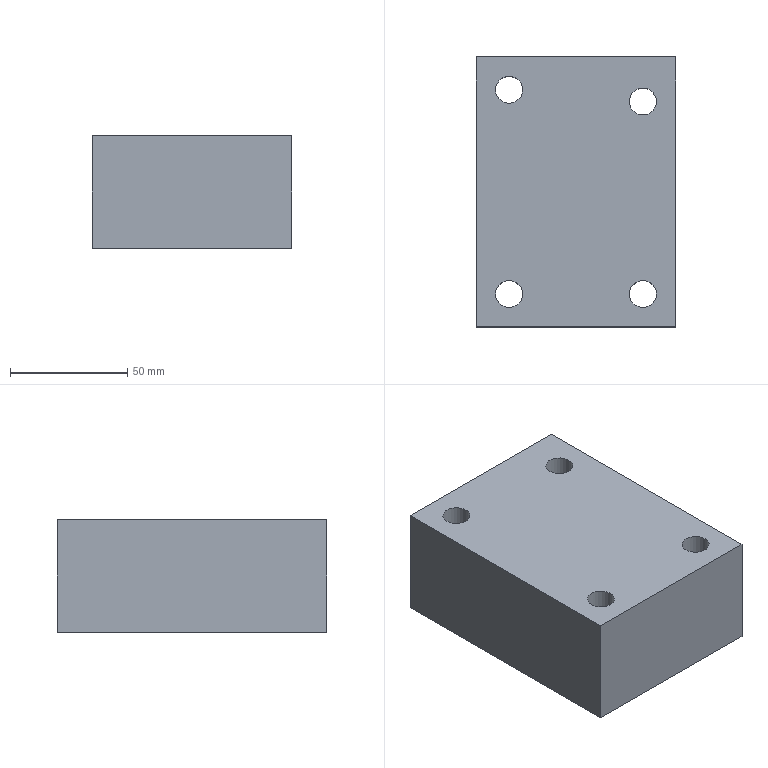Part | NX | features solid 2 | 1 solid | 35 faces | box 85 x 115 x 48 mm | volume 405580 mm3 | cylinder 16 | plane 15 | cone 4 | commonest cylinder face diameters 10 x4 11.509 x4 18.007 x4 8.5 x2 8.506 x2
STEP:
#1=CARTESIAN_POINT('',(1168.789,202.654,50.));
#2=VERTEX_POINT('',#1);
#3=CARTESIAN_POINT('',(1159.786,202.654,50.));
#4=DIRECTION('',(0.,0.,1.));
#5=DIRECTION('',(1.,0.,0.));
#6=AXIS2_PLACEMENT_3D('',#3,#4,#5);
#7=CIRCLE('',#6,9.004);
#8=EDGE_CURVE('',#2,#2,#7,.T.);
#9=ORIENTED_EDGE('',*,*,#8,.T.);
#10=EDGE_LOOP('',(#9));
#11=FACE_BOUND('',#10,.T.);
#12=CARTESIAN_POINT('',(1225.789,115.654,50.));
#13=VERTEX_POINT('',#12);
#14=CARTESIAN_POINT('',(1216.786,115.654,50.));
#15=DIRECTION('',(0.,0.,1.));
#16=DIRECTION('',(1.,0.,0.));
#17=AXIS2_PLACEMENT_3D('',#14,#15,#16);
#18=CIRCLE('',#17,9.004);
#19=EDGE_CURVE('',#13,#13,#18,.T.);
#20=ORIENTED_EDGE('',*,*,#19,.T.);
#21=EDGE_LOOP('',(#20));
#22=FACE_BOUND('',#21,.T.);
#23=CARTESIAN_POINT('',(1230.786,216.654,50.));
#24=VERTEX_POINT('',#23);
#25=CARTESIAN_POINT('',(1145.786,216.654,50.));
#26=VERTEX_POINT('',#25);
#27=CARTESIAN_POINT('',(1188.286,216.654,50.));
#28=DIRECTION('',(-1.,0.,0.));
#29=VECTOR('',#28,1000.);
#30=LINE('',#27,#29);
#31=EDGE_CURVE('',#24,#26,#30,.T.);
#32=ORIENTED_EDGE('',*,*,#31,.F.);
#33=CARTESIAN_POINT('',(1230.786,101.654,50.));
#34=VERTEX_POINT('',#33);
#35=CARTESIAN_POINT('',(1230.786,0.,50.));
#36=DIRECTION('',(0.,-1.,0.));
#37=VECTOR('',#36,1000.);
#38=LINE('',#35,#37);
#39=EDGE_CURVE('',#24,#34,#38,.T.);
#40=ORIENTED_EDGE('',*,*,#39,.T.);
#41=CARTESIAN_POINT('',(1145.786,101.654,50.));
#42=VERTEX_POINT('',#41);
#43=CARTESIAN_POINT('',(1127.,101.654,50.));
#44=DIRECTION('',(-1.,0.,0.));
#45=VECTOR('',#44,1000.);
#46=LINE('',#43,#45);
#47=EDGE_CURVE('',#34,#42,#46,.T.);
#48=ORIENTED_EDGE('',*,*,#47,.T.);
#49=CARTESIAN_POINT('',(1145.786,0.,50.));
#50=DIRECTION('',(0.,1.,0.));
#51=VECTOR('',#50,1000.);
#52=LINE('',#49,#51);
#53=EDGE_CURVE('',#42,#26,#52,.T.);
#54=ORIENTED_EDGE('',*,*,#53,.T.);
#55=EDGE_LOOP('',(#32,#40,#48,#54));
#56=FACE_BOUND('',#55,.T.);
#57=CARTESIAN_POINT('',(1225.789,197.654,50.));
#58=VERTEX_POINT('',#57);
#59=CARTESIAN_POINT('',(1216.786,197.654,50.));
#60=DIRECTION('',(0.,0.,1.));
#61=DIRECTION('',(1.,0.,0.));
#62=AXIS2_PLACEMENT_3D('',#59,#60,#61);
#63=CIRCLE('',#62,9.004);
#64=EDGE_CURVE('',#58,#58,#63,.T.);
#65=ORIENTED_EDGE('',*,*,#64,.T.);
#66=EDGE_LOOP('',(#65));
#67=FACE_BOUND('',#66,.T.);
#68=CARTESIAN_POINT('',(1168.789,115.654,50.));
#69=VERTEX_POINT('',#68);
#70=CARTESIAN_POINT('',(1159.786,115.654,50.));
#71=DIRECTION('',(0.,0.,1.));
#72=DIRECTION('',(1.,0.,0.));
#73=AXIS2_PLACEMENT_3D('',#70,#71,#72);
#74=CIRCLE('',#73,9.004);
#75=EDGE_CURVE('',#69,#69,#74,.T.);
#76=ORIENTED_EDGE('',*,*,#75,.T.);
#77=EDGE_LOOP('',(#76));
#78=FACE_BOUND('',#77,.T.);
#79=CARTESIAN_POINT('',(1156.536,159.154,50.));
#80=VERTEX_POINT('',#79);
#81=CARTESIAN_POINT('',(1160.786,159.154,50.));
#82=DIRECTION('',(0.,0.,-1.));
#83=DIRECTION('',(-1.,0.,0.));
#84=AXIS2_PLACEMENT_3D('',#81,#82,#83);
#85=CIRCLE('',#84,4.25);
#86=EDGE_CURVE('',#80,#80,#85,.T.);
#87=ORIENTED_EDGE('',*,*,#86,.F.);
#88=EDGE_LOOP('',(#87));
#89=FACE_BOUND('',#88,.T.);
#90=CARTESIAN_POINT('',(1211.536,159.154,50.));
#91=VERTEX_POINT('',#90);
#92=CARTESIAN_POINT('',(1215.786,159.154,50.));
#93=DIRECTION('',(0.,0.,-1.));
#94=DIRECTION('',(-1.,0.,0.));
#95=AXIS2_PLACEMENT_3D('',#92,#93,#94);
#96=CIRCLE('',#95,4.25);
#97=EDGE_CURVE('',#91,#91,#96,.T.);
#98=ORIENTED_EDGE('',*,*,#97,.F.);
#99=EDGE_LOOP('',(#98));
#100=FACE_BOUND('',#99,.T.);
#101=CARTESIAN_POINT('',(1206.996,131.014,50.));
#102=VERTEX_POINT('',#101);
#103=CARTESIAN_POINT('',(1199.996,124.014,50.));
#104=VERTEX_POINT('',#103);
#105=CARTESIAN_POINT('',(1203.996,127.014,50.));
#106=DIRECTION('',(0.,0.,-1.));
#107=DIRECTION('',(-1.,0.,0.));
#108=AXIS2_PLACEMENT_3D('',#105,#106,#107);
#109=CIRCLE('',#108,5.);
#110=EDGE_CURVE('',#102,#104,#109,.T.);
#111=ORIENTED_EDGE('',*,*,#110,.F.);
#112=CARTESIAN_POINT('',(1206.996,187.154,50.));
#113=VERTEX_POINT('',#112);
#114=CARTESIAN_POINT('',(1206.996,0.,50.));
#115=DIRECTION('',(0.,1.,0.));
#116=VECTOR('',#115,1000.);
#117=LINE('',#114,#116);
#118=EDGE_CURVE('',#102,#113,#117,.T.);
#119=ORIENTED_EDGE('',*,*,#118,.T.);
#120=CARTESIAN_POINT('',(1199.996,194.154,50.));
#121=VERTEX_POINT('',#120);
#122=CARTESIAN_POINT('',(1203.996,191.154,50.));
#123=DIRECTION('',(0.,0.,-1.));
#124=DIRECTION('',(-1.,0.,0.));
#125=AXIS2_PLACEMENT_3D('',#122,#123,#124);
#126=CIRCLE('',#125,5.);
#127=EDGE_CURVE('',#113,#121,#126,.F.);
#128=ORIENTED_EDGE('',*,*,#127,.T.);
#129=CARTESIAN_POINT('',(1176.576,194.154,50.));
#130=VERTEX_POINT('',#129);
#131=CARTESIAN_POINT('',(1127.,194.154,50.));
#132=DIRECTION('',(-1.,0.,0.));
#133=VECTOR('',#132,1000.);
#134=LINE('',#131,#133);
#135=EDGE_CURVE('',#121,#130,#134,.T.);
#136=ORIENTED_EDGE('',*,*,#135,.T.);
#137=CARTESIAN_POINT('',(1169.576,187.154,50.));
#138=VERTEX_POINT('',#137);
#139=CARTESIAN_POINT('',(1172.576,191.154,50.));
#140=DIRECTION('',(0.,0.,-1.));
#141=DIRECTION('',(-1.,0.,0.));
#142=AXIS2_PLACEMENT_3D('',#139,#140,#141);
#143=CIRCLE('',#142,5.);
#144=EDGE_CURVE('',#138,#130,#143,.T.);
#145=ORIENTED_EDGE('',*,*,#144,.F.);
#146=CARTESIAN_POINT('',(1169.576,131.014,50.));
#147=VERTEX_POINT('',#146);
#148=CARTESIAN_POINT('',(1169.576,0.,50.));
#149=DIRECTION('',(0.,-1.,0.));
#150=VECTOR('',#149,1000.);
#151=LINE('',#148,#150);
#152=EDGE_CURVE('',#138,#147,#151,.T.);
#153=ORIENTED_EDGE('',*,*,#152,.T.);
#154=CARTESIAN_POINT('',(1176.576,124.014,50.));
#155=VERTEX_POINT('',#154);
#156=CARTESIAN_POINT('',(1172.576,127.014,50.));
#157=DIRECTION('',(0.,0.,-1.));
#158=DIRECTION('',(-1.,0.,0.));
#159=AXIS2_PLACEMENT_3D('',#156,#157,#158);
#160=CIRCLE('',#159,5.);
#161=EDGE_CURVE('',#155,#147,#160,.T.);
#162=ORIENTED_EDGE('',*,*,#161,.F.);
#163=CARTESIAN_POINT('',(1127.,124.014,50.));
#164=DIRECTION('',(1.,0.,0.));
#165=VECTOR('',#164,1000.);
#166=LINE('',#163,#165);
#167=EDGE_CURVE('',#155,#104,#166,.T.);
#168=ORIENTED_EDGE('',*,*,#167,.T.);
#169=EDGE_LOOP('',(#111,#119,#128,#136,#145,#153,#162,#168));
#170=FACE_BOUND('',#169,.T.);
#171=CARTESIAN_POINT('',(1127.,0.,50.));
#172=DIRECTION('',(0.,0.,-1.));
#173=DIRECTION('',(-1.,0.,0.));
#174=AXIS2_PLACEMENT_3D('',#171,#172,#173);
#175=PLANE('',#174);
#176=ADVANCED_FACE('',(#11,#22,#56,#67,#78,#89,#100,#170),#175,.T.);
#177=CARTESIAN_POINT('',(1230.786,101.654,98.));
#178=VERTEX_POINT('',#177);
#179=CARTESIAN_POINT('',(1230.786,216.654,98.));
#180=VERTEX_POINT('',#179);
#181=CARTESIAN_POINT('',(1230.786,0.,98.));
#182=DIRECTION('',(0.,1.,0.));
#183=VECTOR('',#182,1000.);
#184=LINE('',#181,#183);
#185=EDGE_CURVE('',#178,#180,#184,.T.);
#186=ORIENTED_EDGE('',*,*,#185,.F.);
#187=CARTESIAN_POINT('',(1230.786,101.654,87.75));
#188=DIRECTION('',(0.,0.,1.));
#189=VECTOR('',#188,1000.);
#190=LINE('',#187,#189);
#191=EDGE_CURVE('',#34,#178,#190,.T.);
#192=ORIENTED_EDGE('',*,*,#191,.F.);
#193=ORIENTED_EDGE('',*,*,#39,.F.);
#194=CARTESIAN_POINT('',(1230.786,216.654,-52.75));
#195=DIRECTION('',(0.,0.,-1.));
#196=VECTOR('',#195,1000.);
#197=LINE('',#194,#196);
#198=EDGE_CURVE('',#180,#24,#197,.T.);
#199=ORIENTED_EDGE('',*,*,#198,.F.);
#200=EDGE_LOOP('',(#186,#192,#193,#199));
#201=FACE_BOUND('',#200,.T.);
#202=CARTESIAN_POINT('',(1230.786,216.654,50.));
#203=DIRECTION('',(1.,0.,0.));
#204=DIRECTION('',(0.,0.,-1.));
#205=AXIS2_PLACEMENT_3D('',#202,#203,#204);
#206=PLANE('',#205);
#207=ADVANCED_FACE('',(#201),#206,.T.);
#208=CARTESIAN_POINT('',(1165.54,202.654,98.));
#209=VERTEX_POINT('',#208);
#210=CARTESIAN_POINT('',(1159.786,202.654,98.));
#211=DIRECTION('',(0.,0.,1.));
#212=DIRECTION('',(1.,0.,0.));
#213=AXIS2_PLACEMENT_3D('',#210,#211,#212);
#214=CIRCLE('',#213,5.755);
#215=EDGE_CURVE('',#209,#209,#214,.T.);
#216=ORIENTED_EDGE('',*,*,#215,.F.);
#217=EDGE_LOOP('',(#216));
#218=FACE_BOUND('',#217,.T.);
#219=CARTESIAN_POINT('',(1165.54,115.654,98.));
#220=VERTEX_POINT('',#219);
#221=CARTESIAN_POINT('',(1159.786,115.654,98.));
#222=DIRECTION('',(0.,0.,1.));
#223=DIRECTION('',(1.,0.,0.));
#224=AXIS2_PLACEMENT_3D('',#221,#222,#223);
#225=CIRCLE('',#224,5.755);
#226=EDGE_CURVE('',#220,#220,#225,.T.);
#227=ORIENTED_EDGE('',*,*,#226,.F.);
#228=EDGE_LOOP('',(#227));
#229=FACE_BOUND('',#228,.T.);
#230=CARTESIAN_POINT('',(1222.54,115.654,98.));
#231=VERTEX_POINT('',#230);
#232=CARTESIAN_POINT('',(1216.786,115.654,98.));
#233=DIRECTION('',(0.,0.,1.));
#234=DIRECTION('',(1.,0.,0.));
#235=AXIS2_PLACEMENT_3D('',#232,#233,#234);
#236=CIRCLE('',#235,5.755);
#237=EDGE_CURVE('',#231,#231,#236,.T.);
#238=ORIENTED_EDGE('',*,*,#237,.F.);
#239=EDGE_LOOP('',(#238));
#240=FACE_BOUND('',#239,.T.);
#241=CARTESIAN_POINT('',(1222.54,197.654,98.));
#242=VERTEX_POINT('',#241);
#243=CARTESIAN_POINT('',(1216.786,197.654,98.));
#244=DIRECTION('',(0.,0.,1.));
#245=DIRECTION('',(1.,0.,0.));
#246=AXIS2_PLACEMENT_3D('',#243,#244,#245);
#247=CIRCLE('',#246,5.755);
#248=EDGE_CURVE('',#242,#242,#247,.T.);
#249=ORIENTED_EDGE('',*,*,#248,.F.);
#250=EDGE_LOOP('',(#249));
#251=FACE_BOUND('',#250,.T.);
#252=CARTESIAN_POINT('',(1145.786,101.654,98.));
#253=VERTEX_POINT('',#252);
#254=CARTESIAN_POINT('',(1188.286,101.654,98.));
#255=DIRECTION('',(-1.,0.,0.));
#256=VECTOR('',#255,1000.);
#257=LINE('',#254,#256);
#258=EDGE_CURVE('',#178,#253,#257,.T.);
#259=ORIENTED_EDGE('',*,*,#258,.F.);
#260=ORIENTED_EDGE('',*,*,#185,.T.);
#261=CARTESIAN_POINT('',(1145.786,216.654,98.));
#262=VERTEX_POINT('',#261);
#263=CARTESIAN_POINT('',(1188.286,216.654,98.));
#264=DIRECTION('',(1.,0.,0.));
#265=VECTOR('',#264,1000.);
#266=LINE('',#263,#265);
#267=EDGE_CURVE('',#262,#180,#266,.T.);
#268=ORIENTED_EDGE('',*,*,#267,.F.);
#269=CARTESIAN_POINT('',(1145.786,0.,98.));
#270=DIRECTION('',(0.,-1.,0.));
#271=VECTOR('',#270,1000.);
#272=LINE('',#269,#271);
#273=EDGE_CURVE('',#262,#253,#272,.T.);
#274=ORIENTED_EDGE('',*,*,#273,.T.);
#275=EDGE_LOOP('',(#259,#260,#268,#274));
#276=FACE_BOUND('',#275,.T.);
#277=CARTESIAN_POINT('',(835.5,0.,98.));
#278=DIRECTION('',(0.,0.,1.));
#279=DIRECTION('',(1.,0.,0.));
#280=AXIS2_PLACEMENT_3D('',#277,#278,#279);
#281=PLANE('',#280);
#282=ADVANCED_FACE('',(#218,#229,#240,#251,#276),#281,.T.);
#283=ORIENTED_EDGE('',*,*,#47,.F.);
#284=ORIENTED_EDGE('',*,*,#191,.T.);
#285=ORIENTED_EDGE('',*,*,#258,.T.);
#286=CARTESIAN_POINT('',(1145.786,101.654,87.75));
#287=DIRECTION('',(0.,0.,-1.));
#288=VECTOR('',#287,1000.);
#289=LINE('',#286,#288);
#290=EDGE_CURVE('',#253,#42,#289,.T.);
#291=ORIENTED_EDGE('',*,*,#290,.T.);
#292=EDGE_LOOP('',(#283,#284,#285,#291));
#293=FACE_BOUND('',#292,.T.);
#294=CARTESIAN_POINT('',(1188.286,101.654,87.75));
#295=DIRECTION('',(0.,-1.,0.));
#296=DIRECTION('',(0.,0.,-1.));
#297=AXIS2_PLACEMENT_3D('',#294,#295,#296);
#298=PLANE('',#297);
#299=ADVANCED_FACE('',(#293),#298,.T.);
#300=ORIENTED_EDGE('',*,*,#267,.T.);
#301=ORIENTED_EDGE('',*,*,#198,.T.);
#302=ORIENTED_EDGE('',*,*,#31,.T.);
#303=CARTESIAN_POINT('',(1145.786,216.654,-52.75));
#304=DIRECTION('',(0.,0.,1.));
#305=VECTOR('',#304,1000.);
#306=LINE('',#303,#305);
#307=EDGE_CURVE('',#26,#262,#306,.T.);
#308=ORIENTED_EDGE('',*,*,#307,.T.);
#309=EDGE_LOOP('',(#300,#301,#302,#308));
#310=FACE_BOUND('',#309,.T.);
#311=CARTESIAN_POINT('',(1188.286,216.654,-52.75));
#312=DIRECTION('',(0.,1.,0.));
#313=DIRECTION('',(0.,0.,1.));
#314=AXIS2_PLACEMENT_3D('',#311,#312,#313);
#315=PLANE('',#314);
#316=ADVANCED_FACE('',(#310),#315,.T.);
#317=ORIENTED_EDGE('',*,*,#273,.F.);
#318=ORIENTED_EDGE('',*,*,#307,.F.);
#319=ORIENTED_EDGE('',*,*,#53,.F.);
#320=ORIENTED_EDGE('',*,*,#290,.F.);
#321=EDGE_LOOP('',(#317,#318,#319,#320));
#322=FACE_BOUND('',#321,.T.);
#323=CARTESIAN_POINT('',(1145.786,216.654,50.));
#324=DIRECTION('',(-1.,0.,0.));
#325=DIRECTION('',(0.,0.,1.));
#326=AXIS2_PLACEMENT_3D('',#323,#324,#325);
#327=PLANE('',#326);
#328=ADVANCED_FACE('',(#322),#327,.T.);
#329=ORIENTED_EDGE('',*,*,#248,.T.);
#330=EDGE_LOOP('',(#329));
#331=FACE_BOUND('',#330,.T.);
#332=CARTESIAN_POINT('',(1222.54,197.654,68.));
#333=VERTEX_POINT('',#332);
#334=CARTESIAN_POINT('',(1216.786,197.654,68.));
#335=DIRECTION('',(0.,0.,1.));
#336=DIRECTION('',(1.,0.,0.));
#337=AXIS2_PLACEMENT_3D('',#334,#335,#336);
#338=CIRCLE('',#337,5.755);
#339=EDGE_CURVE('',#333,#333,#338,.T.);
#340=ORIENTED_EDGE('',*,*,#339,.F.);
#341=EDGE_LOOP('',(#340));
#342=FACE_BOUND('',#341,.T.);
#343=CARTESIAN_POINT('',(1216.786,197.654,45.));
#344=DIRECTION('',(0.,0.,1.));
#345=DIRECTION('',(1.,0.,0.));
#346=AXIS2_PLACEMENT_3D('',#343,#344,#345);
#347=CYLINDRICAL_SURFACE('',#346,5.755);
#348=ADVANCED_FACE('',(#331,#342),#347,.F.);
#349=ORIENTED_EDGE('',*,*,#339,.T.);
#350=EDGE_LOOP('',(#349));
#351=FACE_BOUND('',#350,.T.);
#352=CARTESIAN_POINT('',(1225.789,197.654,68.));
#353=VERTEX_POINT('',#352);
#354=CARTESIAN_POINT('',(1216.786,197.654,68.));
#355=DIRECTION('',(0.,0.,-1.));
#356=DIRECTION('',(1.,0.,0.));
#357=AXIS2_PLACEMENT_3D('',#354,#355,#356);
#358=CIRCLE('',#357,9.004);
#359=EDGE_CURVE('',#353,#353,#358,.F.);
#360=ORIENTED_EDGE('',*,*,#359,.F.);
#361=EDGE_LOOP('',(#360));
#362=FACE_BOUND('',#361,.T.);
#363=CARTESIAN_POINT('',(1216.786,197.654,68.));
#364=DIRECTION('',(0.,0.,1.));
#365=DIRECTION('',(1.,0.,0.));
#366=AXIS2_PLACEMENT_3D('',#363,#364,#365);
#367=PLANE('',#366);
#368=ADVANCED_FACE('',(#351,#362),#367,.F.);
#369=ORIENTED_EDGE('',*,*,#359,.T.);
#370=EDGE_LOOP('',(#369));
#371=FACE_BOUND('',#370,.T.);
#372=ORIENTED_EDGE('',*,*,#64,.F.);
#373=EDGE_LOOP('',(#372));
#374=FACE_BOUND('',#373,.T.);
#375=CARTESIAN_POINT('',(1216.786,197.654,50.));
#376=DIRECTION('',(0.,0.,1.));
#377=DIRECTION('',(1.,0.,0.));
#378=AXIS2_PLACEMENT_3D('',#375,#376,#377);
#379=CYLINDRICAL_SURFACE('',#378,9.004);
#380=ADVANCED_FACE('',(#371,#374),#379,.F.);
#381=ORIENTED_EDGE('',*,*,#237,.T.);
#382=EDGE_LOOP('',(#381));
#383=FACE_BOUND('',#382,.T.);
#384=CARTESIAN_POINT('',(1222.54,115.654,68.));
#385=VERTEX_POINT('',#384);
#386=CARTESIAN_POINT('',(1216.786,115.654,68.));
#387=DIRECTION('',(0.,0.,1.));
#388=DIRECTION('',(1.,0.,0.));
#389=AXIS2_PLACEMENT_3D('',#386,#387,#388);
#390=CIRCLE('',#389,5.755);
#391=EDGE_CURVE('',#385,#385,#390,.T.);
#392=ORIENTED_EDGE('',*,*,#391,.F.);
#393=EDGE_LOOP('',(#392));
#394=FACE_BOUND('',#393,.T.);
#395=CARTESIAN_POINT('',(1216.786,115.654,45.));
#396=DIRECTION('',(0.,0.,1.));
#397=DIRECTION('',(1.,0.,0.));
#398=AXIS2_PLACEMENT_3D('',#395,#396,#397);
#399=CYLINDRICAL_SURFACE('',#398,5.755);
#400=ADVANCED_FACE('',(#383,#394),#399,.F.);
#401=ORIENTED_EDGE('',*,*,#391,.T.);
#402=EDGE_LOOP('',(#401));
#403=FACE_BOUND('',#402,.T.);
#404=CARTESIAN_POINT('',(1225.789,115.654,68.));
#405=VERTEX_POINT('',#404);
#406=CARTESIAN_POINT('',(1216.786,115.654,68.));
#407=DIRECTION('',(0.,0.,-1.));
#408=DIRECTION('',(1.,0.,0.));
#409=AXIS2_PLACEMENT_3D('',#406,#407,#408);
#410=CIRCLE('',#409,9.004);
#411=EDGE_CURVE('',#405,#405,#410,.F.);
#412=ORIENTED_EDGE('',*,*,#411,.F.);
#413=EDGE_LOOP('',(#412));
#414=FACE_BOUND('',#413,.T.);
#415=CARTESIAN_POINT('',(1216.786,115.654,68.));
#416=DIRECTION('',(0.,0.,1.));
#417=DIRECTION('',(1.,0.,0.));
#418=AXIS2_PLACEMENT_3D('',#415,#416,#417);
#419=PLANE('',#418);
#420=ADVANCED_FACE('',(#403,#414),#419,.F.);
#421=ORIENTED_EDGE('',*,*,#411,.T.);
#422=EDGE_LOOP('',(#421));
#423=FACE_BOUND('',#422,.T.);
#424=ORIENTED_EDGE('',*,*,#19,.F.);
#425=EDGE_LOOP('',(#424));
#426=FACE_BOUND('',#425,.T.);
#427=CARTESIAN_POINT('',(1216.786,115.654,50.));
#428=DIRECTION('',(0.,0.,1.));
#429=DIRECTION('',(1.,0.,0.));
#430=AXIS2_PLACEMENT_3D('',#427,#428,#429);
#431=CYLINDRICAL_SURFACE('',#430,9.004);
#432=ADVANCED_FACE('',(#423,#426),#431,.F.);
#433=ORIENTED_EDGE('',*,*,#226,.T.);
#434=EDGE_LOOP('',(#433));
#435=FACE_BOUND('',#434,.T.);
#436=CARTESIAN_POINT('',(1165.54,115.654,68.));
#437=VERTEX_POINT('',#436);
#438=CARTESIAN_POINT('',(1159.786,115.654,68.));
#439=DIRECTION('',(0.,0.,1.));
#440=DIRECTION('',(1.,0.,0.));
#441=AXIS2_PLACEMENT_3D('',#438,#439,#440);
#442=CIRCLE('',#441,5.755);
#443=EDGE_CURVE('',#437,#437,#442,.T.);
#444=ORIENTED_EDGE('',*,*,#443,.F.);
#445=EDGE_LOOP('',(#444));
#446=FACE_BOUND('',#445,.T.);
#447=CARTESIAN_POINT('',(1159.786,115.654,45.));
#448=DIRECTION('',(0.,0.,1.));
#449=DIRECTION('',(1.,0.,0.));
#450=AXIS2_PLACEMENT_3D('',#447,#448,#449);
#451=CYLINDRICAL_SURFACE('',#450,5.755);
#452=ADVANCED_FACE('',(#435,#446),#451,.F.);
#453=ORIENTED_EDGE('',*,*,#443,.T.);
#454=EDGE_LOOP('',(#453));
#455=FACE_BOUND('',#454,.T.);
#456=CARTESIAN_POINT('',(1168.789,115.654,68.));
#457=VERTEX_POINT('',#456);
#458=CARTESIAN_POINT('',(1159.786,115.654,68.));
#459=DIRECTION('',(0.,0.,-1.));
#460=DIRECTION('',(1.,0.,0.));
#461=AXIS2_PLACEMENT_3D('',#458,#459,#460);
#462=CIRCLE('',#461,9.004);
#463=EDGE_CURVE('',#457,#457,#462,.F.);
#464=ORIENTED_EDGE('',*,*,#463,.F.);
#465=EDGE_LOOP('',(#464));
#466=FACE_BOUND('',#465,.T.);
#467=CARTESIAN_POINT('',(1159.786,115.654,68.));
#468=DIRECTION('',(0.,0.,1.));
#469=DIRECTION('',(1.,0.,0.));
#470=AXIS2_PLACEMENT_3D('',#467,#468,#469);
#471=PLANE('',#470);
#472=ADVANCED_FACE('',(#455,#466),#471,.F.);
#473=ORIENTED_EDGE('',*,*,#463,.T.);
#474=EDGE_LOOP('',(#473));
#475=FACE_BOUND('',#474,.T.);
#476=ORIENTED_EDGE('',*,*,#75,.F.);
#477=EDGE_LOOP('',(#476));
#478=FACE_BOUND('',#477,.T.);
#479=CARTESIAN_POINT('',(1159.786,115.654,50.));
#480=DIRECTION('',(0.,0.,1.));
#481=DIRECTION('',(1.,0.,0.));
#482=AXIS2_PLACEMENT_3D('',#479,#480,#481);
#483=CYLINDRICAL_SURFACE('',#482,9.004);
#484=ADVANCED_FACE('',(#475,#478),#483,.F.);
#485=ORIENTED_EDGE('',*,*,#215,.T.);
#486=EDGE_LOOP('',(#485));
#487=FACE_BOUND('',#486,.T.);
#488=CARTESIAN_POINT('',(1165.54,202.654,68.));
#489=VERTEX_POINT('',#488);
#490=CARTESIAN_POINT('',(1159.786,202.654,68.));
#491=DIRECTION('',(0.,0.,1.));
#492=DIRECTION('',(1.,0.,0.));
#493=AXIS2_PLACEMENT_3D('',#490,#491,#492);
#494=CIRCLE('',#493,5.755);
#495=EDGE_CURVE('',#489,#489,#494,.T.);
#496=ORIENTED_EDGE('',*,*,#495,.F.);
#497=EDGE_LOOP('',(#496));
#498=FACE_BOUND('',#497,.T.);
#499=CARTESIAN_POINT('',(1159.786,202.654,45.));
#500=DIRECTION('',(0.,0.,1.));
#501=DIRECTION('',(1.,0.,0.));
#502=AXIS2_PLACEMENT_3D('',#499,#500,#501);
#503=CYLINDRICAL_SURFACE('',#502,5.755);
#504=ADVANCED_FACE('',(#487,#498),#503,.F.);
#505=ORIENTED_EDGE('',*,*,#495,.T.);
#506=EDGE_LOOP('',(#505));
#507=FACE_BOUND('',#506,.T.);
#508=CARTESIAN_POINT('',(1168.789,202.654,68.));
#509=VERTEX_POINT('',#508);
#510=CARTESIAN_POINT('',(1159.786,202.654,68.));
#511=DIRECTION('',(0.,0.,-1.));
#512=DIRECTION('',(1.,0.,0.));
#513=AXIS2_PLACEMENT_3D('',#510,#511,#512);
#514=CIRCLE('',#513,9.004);
#515=EDGE_CURVE('',#509,#509,#514,.F.);
#516=ORIENTED_EDGE('',*,*,#515,.F.);
#517=EDGE_LOOP('',(#516));
#518=FACE_BOUND('',#517,.T.);
#519=CARTESIAN_POINT('',(1159.786,202.654,68.));
#520=DIRECTION('',(0.,0.,1.));
#521=DIRECTION('',(1.,0.,0.));
#522=AXIS2_PLACEMENT_3D('',#519,#520,#521);
#523=PLANE('',#522);
#524=ADVANCED_FACE('',(#507,#518),#523,.F.);
#525=ORIENTED_EDGE('',*,*,#515,.T.);
#526=EDGE_LOOP('',(#525));
#527=FACE_BOUND('',#526,.T.);
#528=ORIENTED_EDGE('',*,*,#8,.F.);
#529=EDGE_LOOP('',(#528));
#530=FACE_BOUND('',#529,.T.);
#531=CARTESIAN_POINT('',(1159.786,202.654,50.));
#532=DIRECTION('',(0.,0.,1.));
#533=DIRECTION('',(1.,0.,0.));
#534=AXIS2_PLACEMENT_3D('',#531,#532,#533);
#535=CYLINDRICAL_SURFACE('',#534,9.004);
#536=ADVANCED_FACE('',(#527,#530),#535,.F.);
#537=CARTESIAN_POINT('',(1156.536,159.154,70.));
#538=VERTEX_POINT('',#537);
#539=CARTESIAN_POINT('',(1160.786,159.154,70.));
#540=DIRECTION('',(0.,0.,-1.));
#541=DIRECTION('',(-1.,0.,0.));
#542=AXIS2_PLACEMENT_3D('',#539,#540,#541);
#543=CIRCLE('',#542,4.25);
#544=EDGE_CURVE('',#538,#538,#543,.F.);
#545=ORIENTED_EDGE('',*,*,#544,.F.);
#546=EDGE_LOOP('',(#545));
#547=FACE_BOUND('',#546,.T.);
#548=CARTESIAN_POINT('',(1160.786,159.154,72.554));
#549=VERTEX_POINT('',#548);
#550=VERTEX_LOOP('',#549);
#551=FACE_BOUND('',#550,.T.);
#552=CARTESIAN_POINT('',(1160.786,159.154,70.));
#553=DIRECTION('',(0.,0.,-1.));
#554=DIRECTION('',(1.,0.,0.));
#555=AXIS2_PLACEMENT_3D('',#552,#553,#554);
#556=CONICAL_SURFACE('',#555,4.25,1.03);
#557=ADVANCED_FACE('',(#547,#551),#556,.F.);
#558=ORIENTED_EDGE('',*,*,#86,.T.);
#559=EDGE_LOOP('',(#558));
#560=FACE_BOUND('',#559,.T.);
#561=ORIENTED_EDGE('',*,*,#544,.T.);
#562=EDGE_LOOP('',(#561));
#563=FACE_BOUND('',#562,.T.);
#564=CARTESIAN_POINT('',(1160.786,159.154,50.));
#565=DIRECTION('',(0.,0.,1.));
#566=DIRECTION('',(-1.,0.,0.));
#567=AXIS2_PLACEMENT_3D('',#564,#565,#566);
#568=CYLINDRICAL_SURFACE('',#567,4.25);
#569=ADVANCED_FACE('',(#560,#563),#568,.F.);
#570=CARTESIAN_POINT('',(1220.036,159.154,70.));
#571=VERTEX_POINT('',#570);
#572=CARTESIAN_POINT('',(1215.786,159.154,70.));
#573=DIRECTION('',(0.,0.,1.));
#574=DIRECTION('',(1.,0.,0.));
#575=AXIS2_PLACEMENT_3D('',#572,#573,#574);
#576=CIRCLE('',#575,4.25);
#577=EDGE_CURVE('',#571,#571,#576,.F.);
#578=ORIENTED_EDGE('',*,*,#577,.T.);
#579=EDGE_LOOP('',(#578));
#580=FACE_BOUND('',#579,.T.);
#581=CARTESIAN_POINT('',(1215.786,159.154,72.554));
#582=VERTEX_POINT('',#581);
#583=VERTEX_LOOP('',#582);
#584=FACE_BOUND('',#583,.T.);
#585=CARTESIAN_POINT('',(1215.786,159.154,70.));
#586=DIRECTION('',(0.,0.,-1.));
#587=DIRECTION('',(-1.,0.,0.));
#588=AXIS2_PLACEMENT_3D('',#585,#586,#587);
#589=CONICAL_SURFACE('',#588,4.25,1.03);
#590=ADVANCED_FACE('',(#580,#584),#589,.F.);
#591=ORIENTED_EDGE('',*,*,#97,.T.);
#592=EDGE_LOOP('',(#591));
#593=FACE_BOUND('',#592,.T.);
#594=ORIENTED_EDGE('',*,*,#577,.F.);
#595=EDGE_LOOP('',(#594));
#596=FACE_BOUND('',#595,.T.);
#597=CARTESIAN_POINT('',(1215.786,159.154,50.));
#598=DIRECTION('',(0.,0.,1.));
#599=DIRECTION('',(1.,0.,0.));
#600=AXIS2_PLACEMENT_3D('',#597,#598,#599);
#601=CYLINDRICAL_SURFACE('',#600,4.25);
#602=ADVANCED_FACE('',(#593,#596),#601,.F.);
#603=CARTESIAN_POINT('',(1206.996,131.014,60.));
#604=VERTEX_POINT('',#603);
#605=CARTESIAN_POINT('',(1206.996,131.014,-87.));
#606=DIRECTION('',(0.,0.,1.));
#607=VECTOR('',#606,1000.);
#608=LINE('',#605,#607);
#609=EDGE_CURVE('',#604,#102,#608,.F.);
#610=ORIENTED_EDGE('',*,*,#609,.F.);
#611=CARTESIAN_POINT('',(1206.996,187.154,60.));
#612=VERTEX_POINT('',#611);
#613=CARTESIAN_POINT('',(1206.996,0.,60.));
#614=DIRECTION('',(0.,1.,0.));
#615=VECTOR('',#614,1000.);
#616=LINE('',#613,#615);
#617=EDGE_CURVE('',#612,#604,#616,.F.);
#618=ORIENTED_EDGE('',*,*,#617,.F.);
#619=CARTESIAN_POINT('',(1206.996,187.154,-87.));
#620=DIRECTION('',(0.,0.,1.));
#621=VECTOR('',#620,1000.);
#622=LINE('',#619,#621);
#623=EDGE_CURVE('',#612,#113,#622,.F.);
#624=ORIENTED_EDGE('',*,*,#623,.T.);
#625=ORIENTED_EDGE('',*,*,#118,.F.);
#626=EDGE_LOOP('',(#610,#618,#624,#625));
#627=FACE_BOUND('',#626,.T.);
#628=CARTESIAN_POINT('',(1206.996,0.,-87.));
#629=DIRECTION('',(-1.,0.,0.));
#630=DIRECTION('',(0.,0.,1.));
#631=AXIS2_PLACEMENT_3D('',#628,#629,#630);
#632=PLANE('',#631);
#633=ADVANCED_FACE('',(#627),#632,.T.);
#634=ORIENTED_EDGE('',*,*,#110,.T.);
#635=CARTESIAN_POINT('',(1199.996,124.014,60.));
#636=VERTEX_POINT('',#635);
#637=CARTESIAN_POINT('',(1199.996,124.014,-87.));
#638=DIRECTION('',(0.,0.,1.));
#639=VECTOR('',#638,1000.);
#640=LINE('',#637,#639);
#641=EDGE_CURVE('',#636,#104,#640,.F.);
#642=ORIENTED_EDGE('',*,*,#641,.F.);
#643=CARTESIAN_POINT('',(1203.996,127.014,60.));
#644=DIRECTION('',(0.,0.,1.));
#645=DIRECTION('',(1.,0.,0.));
#646=AXIS2_PLACEMENT_3D('',#643,#644,#645);
#647=CIRCLE('',#646,5.);
#648=EDGE_CURVE('',#636,#604,#647,.T.);
#649=ORIENTED_EDGE('',*,*,#648,.T.);
#650=ORIENTED_EDGE('',*,*,#609,.T.);
#651=EDGE_LOOP('',(#634,#642,#649,#650));
#652=FACE_BOUND('',#651,.T.);
#653=CARTESIAN_POINT('',(1203.996,127.014,-87.));
#654=DIRECTION('',(0.,0.,1.));
#655=DIRECTION('',(1.,0.,0.));
#656=AXIS2_PLACEMENT_3D('',#653,#654,#655);
#657=CYLINDRICAL_SURFACE('',#656,5.);
#658=ADVANCED_FACE('',(#652),#657,.F.);
#659=CARTESIAN_POINT('',(1176.576,124.014,60.));
#660=VERTEX_POINT('',#659);
#661=CARTESIAN_POINT('',(1176.576,124.014,-87.));
#662=DIRECTION('',(0.,0.,1.));
#663=VECTOR('',#662,1000.);
#664=LINE('',#661,#663);
#665=EDGE_CURVE('',#660,#155,#664,.F.);
#666=ORIENTED_EDGE('',*,*,#665,.F.);
#667=CARTESIAN_POINT('',(268.879,124.014,60.));
#668=DIRECTION('',(1.,0.,0.));
#669=VECTOR('',#668,1000.);
#670=LINE('',#667,#669);
#671=EDGE_CURVE('',#636,#660,#670,.F.);
#672=ORIENTED_EDGE('',*,*,#671,.F.);
#673=ORIENTED_EDGE('',*,*,#641,.T.);
#674=ORIENTED_EDGE('',*,*,#167,.F.);
#675=EDGE_LOOP('',(#666,#672,#673,#674));
#676=FACE_BOUND('',#675,.T.);
#677=CARTESIAN_POINT('',(268.879,124.014,-87.));
#678=DIRECTION('',(0.,1.,0.));
#679=DIRECTION('',(0.,0.,1.));
#680=AXIS2_PLACEMENT_3D('',#677,#678,#679);
#681=PLANE('',#680);
#682=ADVANCED_FACE('',(#676),#681,.T.);
#683=ORIENTED_EDGE('',*,*,#161,.T.);
#684=CARTESIAN_POINT('',(1169.576,131.014,60.));
#685=VERTEX_POINT('',#684);
#686=CARTESIAN_POINT('',(1169.576,131.014,-87.));
#687=DIRECTION('',(0.,0.,1.));
#688=VECTOR('',#687,1000.);
#689=LINE('',#686,#688);
#690=EDGE_CURVE('',#685,#147,#689,.F.);
#691=ORIENTED_EDGE('',*,*,#690,.F.);
#692=CARTESIAN_POINT('',(1172.576,127.014,60.));
#693=DIRECTION('',(0.,0.,1.));
#694=DIRECTION('',(1.,0.,0.));
#695=AXIS2_PLACEMENT_3D('',#692,#693,#694);
#696=CIRCLE('',#695,5.);
#697=EDGE_CURVE('',#685,#660,#696,.T.);
#698=ORIENTED_EDGE('',*,*,#697,.T.);
#699=ORIENTED_EDGE('',*,*,#665,.T.);
#700=EDGE_LOOP('',(#683,#691,#698,#699));
#701=FACE_BOUND('',#700,.T.);
#702=CARTESIAN_POINT('',(1172.576,127.014,-87.));
#703=DIRECTION('',(0.,0.,1.));
#704=DIRECTION('',(1.,0.,0.));
#705=AXIS2_PLACEMENT_3D('',#702,#703,#704);
#706=CYLINDRICAL_SURFACE('',#705,5.);
#707=ADVANCED_FACE('',(#701),#706,.F.);
#708=CARTESIAN_POINT('',(1169.576,187.154,60.));
#709=VERTEX_POINT('',#708);
#710=CARTESIAN_POINT('',(1169.576,187.154,-87.));
#711=DIRECTION('',(0.,0.,1.));
#712=VECTOR('',#711,1000.);
#713=LINE('',#710,#712);
#714=EDGE_CURVE('',#709,#138,#713,.F.);
#715=ORIENTED_EDGE('',*,*,#714,.F.);
#716=CARTESIAN_POINT('',(1169.576,0.,60.));
#717=DIRECTION('',(0.,-1.,0.));
#718=VECTOR('',#717,1000.);
#719=LINE('',#716,#718);
#720=EDGE_CURVE('',#685,#709,#719,.F.);
#721=ORIENTED_EDGE('',*,*,#720,.F.);
#722=ORIENTED_EDGE('',*,*,#690,.T.);
#723=ORIENTED_EDGE('',*,*,#152,.F.);
#724=EDGE_LOOP('',(#715,#721,#722,#723));
#725=FACE_BOUND('',#724,.T.);
#726=CARTESIAN_POINT('',(1169.576,0.,-87.));
#727=DIRECTION('',(1.,0.,0.));
#728=DIRECTION('',(0.,0.,-1.));
#729=AXIS2_PLACEMENT_3D('',#726,#727,#728);
#730=PLANE('',#729);
#731=ADVANCED_FACE('',(#725),#730,.T.);
#732=ORIENTED_EDGE('',*,*,#144,.T.);
#733=CARTESIAN_POINT('',(1176.576,194.154,60.));
#734=VERTEX_POINT('',#733);
#735=CARTESIAN_POINT('',(1176.576,194.154,-87.));
#736=DIRECTION('',(0.,0.,1.));
#737=VECTOR('',#736,1000.);
#738=LINE('',#735,#737);
#739=EDGE_CURVE('',#734,#130,#738,.F.);
#740=ORIENTED_EDGE('',*,*,#739,.F.);
#741=CARTESIAN_POINT('',(1172.576,191.154,60.));
#742=DIRECTION('',(0.,0.,1.));
#743=DIRECTION('',(1.,0.,0.));
#744=AXIS2_PLACEMENT_3D('',#741,#742,#743);
#745=CIRCLE('',#744,5.);
#746=EDGE_CURVE('',#734,#709,#745,.T.);
#747=ORIENTED_EDGE('',*,*,#746,.T.);
#748=ORIENTED_EDGE('',*,*,#714,.T.);
#749=EDGE_LOOP('',(#732,#740,#747,#748));
#750=FACE_BOUND('',#749,.T.);
#751=CARTESIAN_POINT('',(1172.576,191.154,-87.));
#752=DIRECTION('',(0.,0.,1.));
#753=DIRECTION('',(1.,0.,0.));
#754=AXIS2_PLACEMENT_3D('',#751,#752,#753);
#755=CYLINDRICAL_SURFACE('',#754,5.);
#756=ADVANCED_FACE('',(#750),#755,.F.);
#757=CARTESIAN_POINT('',(1199.996,194.154,60.));
#758=VERTEX_POINT('',#757);
#759=CARTESIAN_POINT('',(1199.996,194.154,-87.));
#760=DIRECTION('',(0.,0.,1.));
#761=VECTOR('',#760,1000.);
#762=LINE('',#759,#761);
#763=EDGE_CURVE('',#758,#121,#762,.F.);
#764=ORIENTED_EDGE('',*,*,#763,.F.);
#765=CARTESIAN_POINT('',(268.879,194.154,60.));
#766=DIRECTION('',(-1.,0.,0.));
#767=VECTOR('',#766,1000.);
#768=LINE('',#765,#767);
#769=EDGE_CURVE('',#734,#758,#768,.F.);
#770=ORIENTED_EDGE('',*,*,#769,.F.);
#771=ORIENTED_EDGE('',*,*,#739,.T.);
#772=ORIENTED_EDGE('',*,*,#135,.F.);
#773=EDGE_LOOP('',(#764,#770,#771,#772));
#774=FACE_BOUND('',#773,.T.);
#775=CARTESIAN_POINT('',(268.879,194.154,-87.));
#776=DIRECTION('',(0.,-1.,0.));
#777=DIRECTION('',(0.,0.,-1.));
#778=AXIS2_PLACEMENT_3D('',#775,#776,#777);
#779=PLANE('',#778);
#780=ADVANCED_FACE('',(#774),#779,.T.);
#781=ORIENTED_EDGE('',*,*,#623,.F.);
#782=CARTESIAN_POINT('',(1203.996,191.154,60.));
#783=DIRECTION('',(0.,0.,1.));
#784=DIRECTION('',(1.,0.,0.));
#785=AXIS2_PLACEMENT_3D('',#782,#783,#784);
#786=CIRCLE('',#785,5.);
#787=EDGE_CURVE('',#758,#612,#786,.F.);
#788=ORIENTED_EDGE('',*,*,#787,.F.);
#789=ORIENTED_EDGE('',*,*,#763,.T.);
#790=ORIENTED_EDGE('',*,*,#127,.F.);
#791=EDGE_LOOP('',(#781,#788,#789,#790));
#792=FACE_BOUND('',#791,.T.);
#793=CARTESIAN_POINT('',(1203.996,191.154,-87.));
#794=DIRECTION('',(0.,0.,1.));
#795=DIRECTION('',(1.,0.,0.));
#796=AXIS2_PLACEMENT_3D('',#793,#794,#795);
#797=CYLINDRICAL_SURFACE('',#796,5.);
#798=ADVANCED_FACE('',(#792),#797,.F.);
#799=CARTESIAN_POINT('',(1199.249,183.154,60.));
#800=VERTEX_POINT('',#799);
#801=CARTESIAN_POINT('',(1194.996,183.154,60.));
#802=DIRECTION('',(0.,0.,1.));
#803=DIRECTION('',(1.,0.,0.));
#804=AXIS2_PLACEMENT_3D('',#801,#802,#803);
#805=CIRCLE('',#804,4.253);
#806=EDGE_CURVE('',#800,#800,#805,.T.);
#807=ORIENTED_EDGE('',*,*,#806,.T.);
#808=EDGE_LOOP('',(#807));
#809=FACE_BOUND('',#808,.T.);
#810=CARTESIAN_POINT('',(1184.829,169.154,60.));
#811=VERTEX_POINT('',#810);
#812=CARTESIAN_POINT('',(1180.576,169.154,60.));
#813=DIRECTION('',(0.,0.,1.));
#814=DIRECTION('',(1.,0.,0.));
#815=AXIS2_PLACEMENT_3D('',#812,#813,#814);
#816=CIRCLE('',#815,4.253);
#817=EDGE_CURVE('',#811,#811,#816,.T.);
#818=ORIENTED_EDGE('',*,*,#817,.T.);
#819=EDGE_LOOP('',(#818));
#820=FACE_BOUND('',#819,.T.);
#821=ORIENTED_EDGE('',*,*,#648,.F.);
#822=ORIENTED_EDGE('',*,*,#671,.T.);
#823=ORIENTED_EDGE('',*,*,#697,.F.);
#824=ORIENTED_EDGE('',*,*,#720,.T.);
#825=ORIENTED_EDGE('',*,*,#746,.F.);
#826=ORIENTED_EDGE('',*,*,#769,.T.);
#827=ORIENTED_EDGE('',*,*,#787,.T.);
#828=ORIENTED_EDGE('',*,*,#617,.T.);
#829=EDGE_LOOP('',(#821,#822,#823,#824,#825,#826,#827,#828));
#830=FACE_BOUND('',#829,.T.);
#831=CARTESIAN_POINT('',(1188.286,159.154,60.));
#832=DIRECTION('',(0.,0.,1.));
#833=DIRECTION('',(1.,0.,0.));
#834=AXIS2_PLACEMENT_3D('',#831,#832,#833);
#835=PLANE('',#834);
#836=ADVANCED_FACE('',(#809,#820,#830),#835,.F.);
#837=CARTESIAN_POINT('',(1176.323,169.154,87.753));
#838=VERTEX_POINT('',#837);
#839=CARTESIAN_POINT('',(1180.576,169.154,87.753));
#840=DIRECTION('',(0.,0.,-1.));
#841=DIRECTION('',(-1.,0.,0.));
#842=AXIS2_PLACEMENT_3D('',#839,#840,#841);
#843=CIRCLE('',#842,4.253);
#844=EDGE_CURVE('',#838,#838,#843,.T.);
#845=ORIENTED_EDGE('',*,*,#844,.F.);
#846=EDGE_LOOP('',(#845));
#847=FACE_BOUND('',#846,.T.);
#848=ORIENTED_EDGE('',*,*,#817,.F.);
#849=EDGE_LOOP('',(#848));
#850=FACE_BOUND('',#849,.T.);
#851=CARTESIAN_POINT('',(1180.576,169.154,57.));
#852=DIRECTION('',(0.,0.,1.));
#853=DIRECTION('',(1.,0.,0.));
#854=AXIS2_PLACEMENT_3D('',#851,#852,#853);
#855=CYLINDRICAL_SURFACE('',#854,4.253);
#856=ADVANCED_FACE('',(#847,#850),#855,.F.);
#857=CARTESIAN_POINT('',(1180.576,169.154,92.006));
#858=VERTEX_POINT('',#857);
#859=VERTEX_LOOP('',#858);
#860=FACE_BOUND('',#859,.T.);
#861=ORIENTED_EDGE('',*,*,#844,.T.);
#862=EDGE_LOOP('',(#861));
#863=FACE_BOUND('',#862,.T.);
#864=CARTESIAN_POINT('',(1180.576,169.154,87.753));
#865=DIRECTION('',(0.,0.,-1.));
#866=DIRECTION('',(1.,0.,0.));
#867=AXIS2_PLACEMENT_3D('',#864,#865,#866);
#868=CONICAL_SURFACE('',#867,4.253,0.7854);
#869=ADVANCED_FACE('',(#860,#863),#868,.F.);
#870=CARTESIAN_POINT('',(1190.743,183.154,87.753));
#871=VERTEX_POINT('',#870);
#872=CARTESIAN_POINT('',(1194.996,183.154,87.753));
#873=DIRECTION('',(0.,0.,-1.));
#874=DIRECTION('',(-1.,0.,0.));
#875=AXIS2_PLACEMENT_3D('',#872,#873,#874);
#876=CIRCLE('',#875,4.253);
#877=EDGE_CURVE('',#871,#871,#876,.T.);
#878=ORIENTED_EDGE('',*,*,#877,.F.);
#879=EDGE_LOOP('',(#878));
#880=FACE_BOUND('',#879,.T.);
#881=ORIENTED_EDGE('',*,*,#806,.F.);
#882=EDGE_LOOP('',(#881));
#883=FACE_BOUND('',#882,.T.);
#884=CARTESIAN_POINT('',(1194.996,183.154,57.));
#885=DIRECTION('',(0.,0.,1.));
#886=DIRECTION('',(1.,0.,0.));
#887=AXIS2_PLACEMENT_3D('',#884,#885,#886);
#888=CYLINDRICAL_SURFACE('',#887,4.253);
#889=ADVANCED_FACE('',(#880,#883),#888,.F.);
#890=CARTESIAN_POINT('',(1194.996,183.154,92.006));
#891=VERTEX_POINT('',#890);
#892=VERTEX_LOOP('',#891);
#893=FACE_BOUND('',#892,.T.);
#894=ORIENTED_EDGE('',*,*,#877,.T.);
#895=EDGE_LOOP('',(#894));
#896=FACE_BOUND('',#895,.T.);
#897=CARTESIAN_POINT('',(1194.996,183.154,87.753));
#898=DIRECTION('',(0.,0.,-1.));
#899=DIRECTION('',(1.,0.,0.));
#900=AXIS2_PLACEMENT_3D('',#897,#898,#899);
#901=CONICAL_SURFACE('',#900,4.253,0.7854);
#902=ADVANCED_FACE('',(#893,#896),#901,.F.);
#903=CLOSED_SHELL('',(#176,#207,#282,#299,#316,#328,#348,#368,#380,#400,#420,#432,#452,#472,#484,#504,#524,#536,#557,#569,#590,#602,#633,#658,#682,#707,#731,#756,#780,#798,#836,#856,#869,#889,#902));
#904=MANIFOLD_SOLID_BREP('',#903);
#905=(LENGTH_UNIT()NAMED_UNIT(*)SI_UNIT(.MILLI.,.METRE.));
#906=UNCERTAINTY_MEASURE_WITH_UNIT(LENGTH_MEASURE(0.00001),#905,'','');
#907=(NAMED_UNIT(*)PLANE_ANGLE_UNIT()SI_UNIT($,.RADIAN.));
#908=(NAMED_UNIT(*)SI_UNIT($,.STERADIAN.)SOLID_ANGLE_UNIT());
#909=(GEOMETRIC_REPRESENTATION_CONTEXT(3)GLOBAL_UNCERTAINTY_ASSIGNED_CONTEXT((#906))GLOBAL_UNIT_ASSIGNED_CONTEXT((#905,#907,#908))REPRESENTATION_CONTEXT('',''));
#910=ADVANCED_BREP_SHAPE_REPRESENTATION('',(#904),#909);